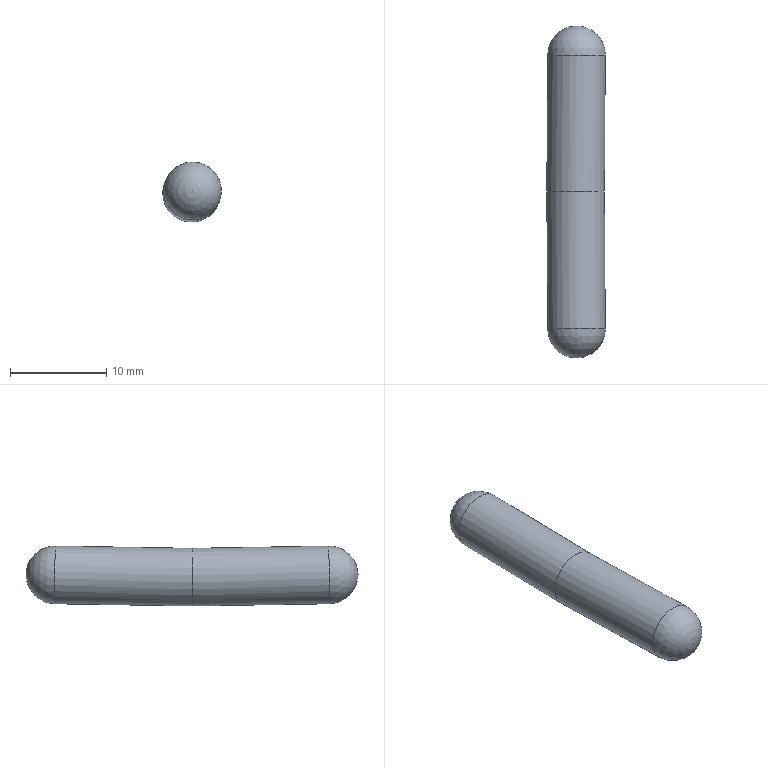Part | NX | features solid 2 | 1 solid | 4 faces | box 6.099 x 34.468 x 6.24 mm | volume 918.133 mm3 | cylinder 2 | sphere 2 | commonest cylinder face diameters 6 x2
STEP:
#1=CARTESIAN_POINT('',(0.09807,14.183,18.625));
#2=VERTEX_POINT('',#1);
#3=CARTESIAN_POINT('',(0.09807,14.234,15.626));
#4=DIRECTION('',(0.006922,0.9998,0.01681));
#5=DIRECTION('',(0.,-0.01681,0.9999));
#6=AXIS2_PLACEMENT_3D('',#3,#4,#5);
#7=CIRCLE('',#6,3.);
#8=EDGE_CURVE('',#2,#2,#7,.T.);
#9=ORIENTED_EDGE('',*,*,#8,.F.);
#10=EDGE_LOOP('',(#9));
#11=FACE_BOUND('',#10,.T.);
#12=CARTESIAN_POINT('',(-1.143,0.,12.612));
#13=VERTEX_POINT('',#12);
#14=CARTESIAN_POINT('',(-0.0004823,0.,15.387));
#15=DIRECTION('',(0.,1.,0.));
#16=DIRECTION('',(-0.3808,0.,-0.9247));
#17=AXIS2_PLACEMENT_3D('',#14,#15,#16);
#18=ELLIPSE('',#17,3.,3.);
#19=EDGE_CURVE('',#13,#13,#18,.T.);
#20=ORIENTED_EDGE('',*,*,#19,.T.);
#21=EDGE_LOOP('',(#20));
#22=FACE_BOUND('',#21,.T.);
#23=CARTESIAN_POINT('',(0.004771,0.7587,15.399));
#24=DIRECTION('',(-0.006922,-0.9998,-0.01681));
#25=DIRECTION('',(0.,-0.01681,0.9999));
#26=AXIS2_PLACEMENT_3D('',#23,#24,#25);
#27=CYLINDRICAL_SURFACE('',#26,3.);
#28=ADVANCED_FACE('',(#11,#22),#27,.T.);
#29=ORIENTED_EDGE('',*,*,#8,.T.);
#30=EDGE_LOOP('',(#29));
#31=FACE_BOUND('',#30,.T.);
#32=CARTESIAN_POINT('',(0.09807,14.234,15.626));
#33=DIRECTION('',(-0.006922,-0.9998,-0.01681));
#34=DIRECTION('',(0.,-0.01681,0.9999));
#35=AXIS2_PLACEMENT_3D('',#32,#33,#34);
#36=SPHERICAL_SURFACE('',#35,3.);
#37=ADVANCED_FACE('',(#31),#36,.T.);
#38=CARTESIAN_POINT('',(0.09807,-14.183,18.625));
#39=VERTEX_POINT('',#38);
#40=CARTESIAN_POINT('',(0.09807,-14.234,15.626));
#41=DIRECTION('',(-0.006922,0.9998,-0.01681));
#42=DIRECTION('',(0.,0.01681,0.9999));
#43=AXIS2_PLACEMENT_3D('',#40,#41,#42);
#44=CIRCLE('',#43,3.);
#45=EDGE_CURVE('',#39,#39,#44,.T.);
#46=ORIENTED_EDGE('',*,*,#45,.T.);
#47=EDGE_LOOP('',(#46));
#48=FACE_BOUND('',#47,.T.);
#49=ORIENTED_EDGE('',*,*,#19,.F.);
#50=EDGE_LOOP('',(#49));
#51=FACE_BOUND('',#50,.T.);
#52=CARTESIAN_POINT('',(0.004771,-0.7587,15.399));
#53=DIRECTION('',(-0.006922,0.9998,-0.01681));
#54=DIRECTION('',(0.,0.01681,0.9999));
#55=AXIS2_PLACEMENT_3D('',#52,#53,#54);
#56=CYLINDRICAL_SURFACE('',#55,3.);
#57=ADVANCED_FACE('',(#48,#51),#56,.T.);
#58=ORIENTED_EDGE('',*,*,#45,.F.);
#59=EDGE_LOOP('',(#58));
#60=FACE_BOUND('',#59,.T.);
#61=CARTESIAN_POINT('',(0.09807,-14.234,15.626));
#62=DIRECTION('',(-0.006922,0.9998,-0.01681));
#63=DIRECTION('',(0.,0.01681,0.9999));
#64=AXIS2_PLACEMENT_3D('',#61,#62,#63);
#65=SPHERICAL_SURFACE('',#64,3.);
#66=ADVANCED_FACE('',(#60),#65,.T.);
#67=CLOSED_SHELL('',(#28,#37,#57,#66));
#68=MANIFOLD_SOLID_BREP('',#67);
#69=(LENGTH_UNIT()NAMED_UNIT(*)SI_UNIT(.MILLI.,.METRE.));
#70=UNCERTAINTY_MEASURE_WITH_UNIT(LENGTH_MEASURE(0.00001),#69,'','');
#71=(NAMED_UNIT(*)PLANE_ANGLE_UNIT()SI_UNIT($,.RADIAN.));
#72=(NAMED_UNIT(*)SI_UNIT($,.STERADIAN.)SOLID_ANGLE_UNIT());
#73=(GEOMETRIC_REPRESENTATION_CONTEXT(3)GLOBAL_UNCERTAINTY_ASSIGNED_CONTEXT((#70))GLOBAL_UNIT_ASSIGNED_CONTEXT((#69,#71,#72))REPRESENTATION_CONTEXT('',''));
#74=ADVANCED_BREP_SHAPE_REPRESENTATION('',(#68),#73);